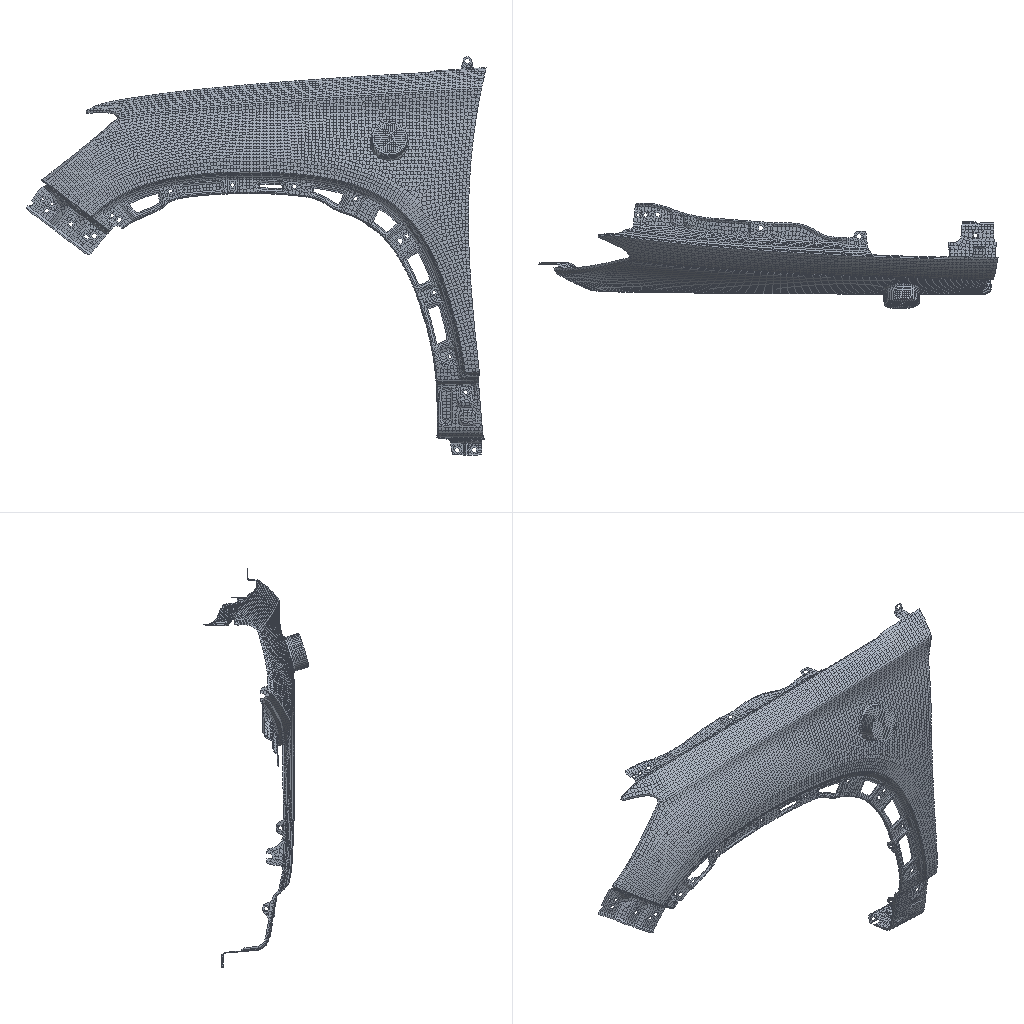Simulation study | abaqus
Set-up summary:
category,name,step,type,value,unit,region
solver,abaqus
solver,version,,,Abaqus/Standard 3DEXPERIENCE R2017x
units,not stated in the deck,,not stated
analysis,deck,,static,static
load_step,load,load,static,nlgeom=True
load_step,unload,unload,static,nlgeom=True
contact,interactions,,,general=0 pairs=1 ties=0
load_step,requested,,,2
mesh,nodes,,,12250
mesh,elements,,,11562
element_type,S3,,shell,568
element_type,S4,,shell,9090
element_type,C3D8,,solid,1664
element_type,C3D8H,,solid,240
load,load commands in deck,,count,1
bc,support commands in deck,,count,14
material,HC180Y,,in results
material,MAT-STEEL,,in results
material,RUBBER,,in results
check,setup vs results,,match,"per instance, exact: element labels, types and connectivity; labels of the nodes the elements use; coordinates not compared"
Abaqus input file, long lists of numbers shortened:
**
** ABAQUS Input Deck Generated by HyperMesh Version  : 14.0.0.88
** Generated using HyperMesh-Abaqus Template Version : 14.0
**
**   Template:  ABAQUS/STANDARD 3D
**
*NODE
         1,  -435.848       ,  -889.15        ,  300.419
         2,  -437.816       ,  -889.15        ,  297.793
** (12247 more lines like these left out)
**HMNAME SYSTEMCOL auto1,         1,    4
*SYSTEM
317.799, -956.623, 508.703, 316.8, -956.657 , 508.745
317.83, -956.33, 509.658
*NODE, SYSTEM=R
   2133045,  0.0            ,  0.0            ,  0.0
**HWCOLOR COMP        371    21
*ELEMENT,TYPE=S3,ELSET=KX63_F08-8403101_HC180Y_T070
        13,        27,      3741,      2715
        37,      7291,      7290,       590
** (566 more lines like these left out)
**HWCOLOR COMP        371    21
*ELEMENT,TYPE=S4,ELSET=KX63_F08-8403101_HC180Y_T070
         1,         4,         5,         6,         3
         2,       581,       611,        31,       588
** (9088 more lines like these left out)
**HWCOLOR COMP          1    21
*ELEMENT,TYPE=C3D8,ELSET=impactor
   2127998,    839956,    839918,    839973,    839922,    839778,    839312,    839786,
    839315
** (3326 more lines like these left out)
**HWCOLOR COMP          2    55
*ELEMENT,TYPE=C3D8H,ELSET=rubber
     14376,    838547,    838651,    838694,    838463,    838914,    838951,    839220,
    838890
** (478 more lines like these left out)
**HWNAME COMP    2000070 FRONT_RH_REB2
**HWCOLOR COMP    2000070    29
*KINEMATIC COUPLING,REF NODE=2133045
    838213,1,6
    838215,1,6
    838216,1,6
    838220,1,6
    838224,1,6
    838230,1,6
    838236,1,6
    838237,1,6
    838238,1,6
    838239,1,6
    838242,1,6
    838244,1,6
    838247,1,6
    838248,1,6
    838250,1,6
    838251,1,6
    838252,1,6
    838253,1,6
    838256,1,6
    838257,1,6
    838259,1,6
    838260,1,6
    838272,1,6
    838275,1,6
    838278,1,6
    838282,1,6
    838284,1,6
    838299,1,6
    838301,1,6
    838302,1,6
    838305,1,6
    838307,1,6
    838308,1,6
    838313,1,6
    838315,1,6
    838319,1,6
    838320,1,6
    838321,1,6
    838324,1,6
    838325,1,6
** (224 more lines like these left out)
**HWNAME COMP        370 RB2
**HWCOLOR COMP        370    18
*COUPLING, REF NODE=839102, CONSTRAINT NAME="HM_coupkin_20971", SURFACE="HM_coupkin_surface_20971"
*KINEMATIC
1,6
*SURFACE, NAME ="HM_coupkin_surface_20971", TYPE = NODE
       349, 1
       350, 1
      6702, 1
      6704, 1
      6707, 1
      6709, 1
      6712, 1
      6714, 1
     11735, 1
     11737, 1
     11738, 1
     11741, 1
     11743, 1
     11744, 1
     11754, 1
     11837, 1
     11869, 1
     11870, 1
     11879, 1
     12733, 1
**HWNAME COMP        370 RB2
**HWCOLOR COMP        370    18
*COUPLING, REF NODE=839103, CONSTRAINT NAME="HM_coupkin_20972", SURFACE="HM_coupkin_surface_20972"
*KINEMATIC
1,6
*SURFACE, NAME ="HM_coupkin_surface_20972", TYPE = NODE
       321, 1
       322, 1
      6671, 1
      6678, 1
     12483, 1
     12560, 1
     12561, 1
     12562, 1
     12563, 1
     12568, 1
     12569, 1
     12573, 1
     12574, 1
     12575, 1
     12584, 1
     12585, 1
     12591, 1
     12593, 1
     12600, 1
     12611, 1
**HWNAME COMP        370 RB2
**HWCOLOR COMP        370    18
*COUPLING, REF NODE=839104, CONSTRAINT NAME="HM_coupkin_20973", SURFACE="HM_coupkin_surface_20973"
*KINEMATIC
1,6
*SURFACE, NAME ="HM_coupkin_surface_20973", TYPE = NODE
      7110, 1
      7113, 1
      7118, 1
      7119, 1
      7129, 1
**HWNAME COMP        370 RB2
**HWCOLOR COMP        370    18
*COUPLING, REF NODE=839105, CONSTRAINT NAME="HM_coupkin_20974", SURFACE="HM_coupkin_surface_20974"
*KINEMATIC
1,6
*SURFACE, NAME ="HM_coupkin_surface_20974", TYPE = NODE
     11441, 1
     11445, 1
     11446, 1
     11448, 1
     11451, 1
**HWNAME COMP        370 RB2
**HWCOLOR COMP        370    18
*COUPLING, REF NODE=839106, CONSTRAINT NAME="HM_coupkin_20976", SURFACE="HM_coupkin_surface_20976"
*KINEMATIC
1,6
*SURFACE, NAME ="HM_coupkin_surface_20976", TYPE = NODE
      7300, 1
      7326, 1
      7330, 1
      7331, 1
      7333, 1
      7334, 1
      7335, 1
      7337, 1
     11729, 1
     11749, 1
     11751, 1
     11755, 1
     11756, 1
     11757, 1
     11771, 1
     12043, 1
     12068, 1
     12111, 1
     12116, 1
     12220, 1
**HWNAME COMP        370 RB2
**HWCOLOR COMP        370    18
*COUPLING, REF NODE=839108, CONSTRAINT NAME="HM_coupkin_20983", SURFACE="HM_coupkin_surface_20983"
*KINEMATIC
1,6
*SURFACE, NAME ="HM_coupkin_surface_20983", TYPE = NODE
        36, 1
        49, 1
        78, 1
        80, 1
        81, 1
        82, 1
        85, 1
        91, 1
       105, 1
       107, 1
      7750, 1
      7761, 1
     11457, 1
     11458, 1
     11460, 1
     11461, 1
     11462, 1
     11463, 1
     11464, 1
     11588, 1
    839107, 1
**HWNAME COMP        370 RB2
**HWCOLOR COMP        370    18
*COUPLING, REF NODE=839109, CONSTRAINT NAME="HM_coupkin_20984", SURFACE="HM_coupkin_surface_20984"
*KINEMATIC
1,6
*SURFACE, NAME ="HM_coupkin_surface_20984", TYPE = NODE
      7612, 1
      7613, 1
      7630, 1
     12349, 1
     12580, 1
     12581, 1
     12587, 1
     12588, 1
     12596, 1
     12598, 1
     12601, 1
     12602, 1
     12603, 1
     12604, 1
     12605, 1
     12606, 1
     12607, 1
     12608, 1
     12609, 1
     12610, 1
**HWNAME COMP        370 RB2
**HWCOLOR COMP        370    18
*COUPLING, REF NODE=839110, CONSTRAINT NAME="HM_coupkin_20985", SURFACE="HM_coupkin_surface_20985"
*KINEMATIC
1,6
*SURFACE, NAME ="HM_coupkin_surface_20985", TYPE = NODE
      7451, 1
      7458, 1
     12511, 1
     12514, 1
     12519, 1
     12524, 1
     12525, 1
     12530, 1
     12531, 1
     12536, 1
     12541, 1
     12543, 1
     12546, 1
     12548, 1
     12552, 1
     12553, 1
     12557, 1
     12558, 1
     12576, 1
     12577, 1
**HWNAME COMP        370 RB2
**HWCOLOR COMP        370    18
*COUPLING, REF NODE=839111, CONSTRAINT NAME="HM_coupkin_20986", SURFACE="HM_coupkin_surface_20986"
*KINEMATIC
1,6
*SURFACE, NAME ="HM_coupkin_surface_20986", TYPE = NODE
       675, 1
       677, 1
       678, 1
       682, 1
     12430, 1
     12431, 1
     12435, 1
     12436, 1
     12441, 1
     12442, 1
     12444, 1
     12445, 1
     12446, 1
     12447, 1
     12448, 1
     12449, 1
**HWNAME COMP        370 RB2
**HWCOLOR COMP        370    18
*COUPLING, REF NODE=839144, CONSTRAINT NAME="HM_coupkin_21050", SURFACE="HM_coupkin_surface_21050"
*KINEMATIC
1,6
*SURFACE, NAME ="HM_coupkin_surface_21050", TYPE = NODE
       977, 1
       978, 1
       979, 1
       984, 1
       995, 1
       996, 1
       998, 1
      1018, 1
     12451, 1
     12452, 1
     12453, 1
     12454, 1
     12455, 1
     12456, 1
     12457, 1
     12458, 1
**HWNAME COMP        370 RB2
**HWCOLOR COMP        370    18
*COUPLING, REF NODE=839145, CONSTRAINT NAME="HM_coupkin_21051", SURFACE="HM_coupkin_surface_21051"
*KINEMATIC
1,6
*SURFACE, NAME ="HM_coupkin_surface_21051", TYPE = NODE
       883, 1
       888, 1
       889, 1
       893, 1
       895, 1
       896, 1
       898, 1
       900, 1
       902, 1
       903, 1
       906, 1
       907, 1
       909, 1
       910, 1
       914, 1
     11727, 1
     11775, 1
     11781, 1
     12460, 1
     12463, 1
**HWNAME COMP        370 RB2
**HWCOLOR COMP        370    18
*COUPLING, REF NODE=839146, CONSTRAINT NAME="HM_coupkin_21052", SURFACE="HM_coupkin_surface_21052"
*KINEMATIC
1,6
*SURFACE, NAME ="HM_coupkin_surface_21052", TYPE = NODE
       997, 1
      1008, 1
      1016, 1
      1021, 1
     12078, 1
     12079, 1
     12459, 1
     12461, 1
     12462, 1
     12467, 1
     12468, 1
     12469, 1
**HMNAME SYSTEMCOL auto1,         1,    4
*TRANSFORM, TYPE=R, NSET=HM_auto_transform_208C35
-0.9985, -0.03403, 0.04269,  0.03089,  0.2926,  0.9557
**HMORIENT ORIGIN  317.799,-956.623,508.703
**HM_PROP_ID         38
**HM_comp_by_property "impactor"    56
*SOLID SECTION, ELSET=impactor, MATERIAL=mat-steel
**HM_PROP_ID         39
**HM_comp_by_property "rubber"    56
*SOLID SECTION, ELSET=rubber, MATERIAL=rubber
**HM_PROP_ID         25
**HM_comp_by_property "KX63_F08-8403101_HC180Y_T070"     4
*SHELL SECTION, ELSET=KX63_F08-8403101_HC180Y_T070, MATERIAL=HC180Y
0.7       ,
*ELSET, ELSET=master
      3345,      3351,      3357,      3363,      3367,      3373,      3380,      3387,
      3394,      3401,      3408,      3415,      3422,      3429,      9700,      9732,
** (19 more lines like these left out)
*NSET, NSET=node
   2133045,
*NSET, NSET=HM_auto_transform_208C35
   2133045,
**HMNAME MATS          2 HC180Y     3
*MATERIAL, NAME=HC180Y
*DENSITY
7.8500E-09,0.0
*ELASTIC, TYPE = ISOTROPIC
210000.0  ,0.3       ,0.0
*PLASTIC
239.2     ,0.0       ,0.0
260.6     ,0.0092    ,0.0
281.1     ,0.0149    ,0.0
310.0     ,0.03      ,0.0
329.1     ,0.0431    ,0.0
346.0     ,0.0575    ,0.0
361.8     ,0.074     ,0.0
374.9     ,0.0907    ,0.0
390.9     ,0.115     ,0.0
405.6     ,0.1426    ,0.0
416.3     ,0.1661    ,0.0
423.2     ,0.183     ,0.0
432.6     ,0.2086    ,0.0
439.3     ,0.2298    ,0.0
442.9     ,0.2487    ,0.0
**HMNAME MATS          3 mat-steel     4
*MATERIAL, NAME=mat-steel
*DENSITY
7.8500E-09,0.0
*ELASTIC, TYPE = ISOTROPIC
210000.0  ,0.3       ,0.0
**HMNAME MATS        115 rubber     5
*MATERIAL, NAME=rubber
*DENSITY
1.0000E-09,0.0
*HYPERELASTIC, N = 2,POLYNOMIAL
0.3559   ,-0.2859  ,1.354    ,0.   ,0.   ,0.   ,0.   ,
**HMNAME PROPERTY         40 FRIC
*SURFACE INTERACTION, NAME = FRIC
*FRICTION
0.2       ,0.0       ,0.0       ,0.0
**HMNAME GROUPS          3 cp
*CONTACT PAIR, INTERACTION=FRIC, ADJUST=0.05, TYPE=SURFACE TO SURFACE
slave, master
*SURFACE, NAME = master, TYPE = ELEMENT
master,SNEG
*SURFACE, NAME = slave, TYPE = ELEMENT
     14376, S2
     14377, S2
    810251, S2
     14378, S2
     14379, S2
     14380, S2
     14385, S2
    810296, S2
     14381, S2
    810252, S2
     14417, S2
     14382, S2
     14387, S2
    810253, S2
     14383, S2
     14384, S2
     14391, S2
     14386, S2
     14388, S2
     14422, S2
     14389, S2
     14390, S2
    810287, S2
     14392, S2
     14496, S2
     14393, S2
     14394, S2
    810267, S2
     14395, S2
     14396, S2
     14397, S2
     14398, S2
     14399, S2
    810254, S2
     14400, S2
     14401, S2
    810255, S2
     14476, S2
     21055, S2
     14402, S2
** (200 more lines like these left out)
**HWNAME LOADCOL          1 spc
**HWCOLOR LOADCOL          1    18
*BOUNDARY
    839111,1,6,
    839110,1,6,
    839102,1,6,
    839103,1,6,
    839106,1,6,
    839108,1,6,
    839146,1,6,
    839144,1,6,
    839109,1,6,
    839145,1,6,
    839105,1,6,
    839104,1,6,
   2133045,1,2,
   2133045,4,6,
**HMNAME LOADSTEP          1 load
*STEP, NAME = load, NLGEOM = YES
*STATIC
0.1       ,1.0       ,1.0000E-06,0.2
*MONITOR, DOF =     3, NODE = node
**HWNAME LOADCOL          2 load
**HWCOLOR LOADCOL          2     6
*CLOAD
   2133045,3,400.0
*OUTPUT, FIELD
*NODE OUTPUT
U,
CF,
*ELEMENT OUTPUT
S,
E,
PEEQ,
*END STEP
**HMNAME LOADSTEP          2 unload
*STEP, NAME = unload, NLGEOM = YES
*STATIC
0.1       ,1.0       ,1.0000E-06,0.2
*MONITOR, DOF =     3, NODE = node
**HWNAME LOADCOL          3 unload
**HWCOLOR LOADCOL          3     6
*CLOAD, OP=NEW
*OUTPUT, FIELD
*NODE OUTPUT
U,
CF,
*ELEMENT OUTPUT
S,
E,
PEEQ,
*END STEP
*****
Results summary:
result,step,,completed,increments=7 time=1.0/1.0
result,step,,completed,increments=7 time=1.0/1.0
result,analysis,,,static
result,last_loadstep,,,2
result,analysis steps,,count,2
result,primary field,,,"U, UR"